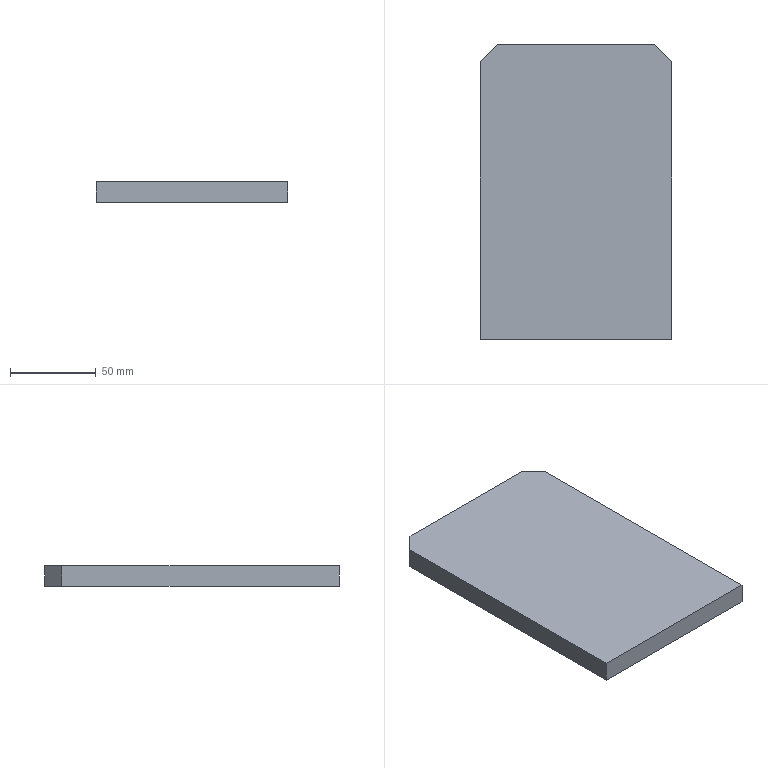Part | SolidWorks | features BaseBody 1 | 1 solid | 8 faces | box 112 x 172 x 12 mm | volume 229968 mm3 | plane 8
STEP:
#1=CARTESIAN_POINT('',(56.,-84.5,-6.));
#2=VERTEX_POINT('',#1);
#3=CARTESIAN_POINT('',(56.,-84.5,6.));
#4=VERTEX_POINT('',#3);
#5=CARTESIAN_POINT('',(56.,-84.5,6.));
#6=DIRECTION('',(0.,0.,1.));
#7=VECTOR('',#6,1000.);
#8=LINE('',#5,#7);
#9=EDGE_CURVE('',#2,#4,#8,.T.);
#10=ORIENTED_EDGE('',*,*,#9,.F.);
#11=CARTESIAN_POINT('',(56.,77.5,-6.));
#12=VERTEX_POINT('',#11);
#13=CARTESIAN_POINT('',(56.,77.5,-6.));
#14=DIRECTION('',(0.,1.,0.));
#15=VECTOR('',#14,1000.);
#16=LINE('',#13,#15);
#17=EDGE_CURVE('',#2,#12,#16,.T.);
#18=ORIENTED_EDGE('',*,*,#17,.T.);
#19=CARTESIAN_POINT('',(56.,77.5,6.));
#20=VERTEX_POINT('',#19);
#21=CARTESIAN_POINT('',(56.,77.5,6.));
#22=DIRECTION('',(0.,0.,-1.));
#23=VECTOR('',#22,1000.);
#24=LINE('',#21,#23);
#25=EDGE_CURVE('',#20,#12,#24,.T.);
#26=ORIENTED_EDGE('',*,*,#25,.F.);
#27=CARTESIAN_POINT('',(56.,77.5,6.));
#28=DIRECTION('',(0.,1.,0.));
#29=VECTOR('',#28,1000.);
#30=LINE('',#27,#29);
#31=EDGE_CURVE('',#4,#20,#30,.T.);
#32=ORIENTED_EDGE('',*,*,#31,.F.);
#33=EDGE_LOOP('',(#10,#18,#26,#32));
#34=FACE_OUTER_BOUND('',#33,.T.);
#35=CARTESIAN_POINT('',(56.,77.5,6.));
#36=DIRECTION('',(-1.,0.,0.));
#37=DIRECTION('',(0.,-1.,0.));
#38=AXIS2_PLACEMENT_3D('',#35,#36,#37);
#39=PLANE('',#38);
#40=ADVANCED_FACE('',(#34),#39,.F.);
#41=CARTESIAN_POINT('',(-56.,-84.5,6.));
#42=VERTEX_POINT('',#41);
#43=CARTESIAN_POINT('',(-56.,-84.5,-6.));
#44=VERTEX_POINT('',#43);
#45=CARTESIAN_POINT('',(-56.,-84.5,6.));
#46=DIRECTION('',(0.,0.,-1.));
#47=VECTOR('',#46,1000.);
#48=LINE('',#45,#47);
#49=EDGE_CURVE('',#42,#44,#48,.T.);
#50=ORIENTED_EDGE('',*,*,#49,.F.);
#51=CARTESIAN_POINT('',(-56.,77.5,6.));
#52=VERTEX_POINT('',#51);
#53=CARTESIAN_POINT('',(-56.,77.5,6.));
#54=DIRECTION('',(0.,-1.,0.));
#55=VECTOR('',#54,1000.);
#56=LINE('',#53,#55);
#57=EDGE_CURVE('',#52,#42,#56,.T.);
#58=ORIENTED_EDGE('',*,*,#57,.F.);
#59=CARTESIAN_POINT('',(-56.,77.5,-6.));
#60=VERTEX_POINT('',#59);
#61=CARTESIAN_POINT('',(-56.,77.5,6.));
#62=DIRECTION('',(0.,0.,-1.));
#63=VECTOR('',#62,1000.);
#64=LINE('',#61,#63);
#65=EDGE_CURVE('',#52,#60,#64,.T.);
#66=ORIENTED_EDGE('',*,*,#65,.T.);
#67=CARTESIAN_POINT('',(-56.,77.5,-6.));
#68=DIRECTION('',(0.,-1.,0.));
#69=VECTOR('',#68,1000.);
#70=LINE('',#67,#69);
#71=EDGE_CURVE('',#60,#44,#70,.T.);
#72=ORIENTED_EDGE('',*,*,#71,.T.);
#73=EDGE_LOOP('',(#50,#58,#66,#72));
#74=FACE_OUTER_BOUND('',#73,.T.);
#75=CARTESIAN_POINT('',(-56.,77.5,6.));
#76=DIRECTION('',(1.,0.,0.));
#77=DIRECTION('',(0.,1.,0.));
#78=AXIS2_PLACEMENT_3D('',#75,#76,#77);
#79=PLANE('',#78);
#80=ADVANCED_FACE('',(#74),#79,.F.);
#81=ORIENTED_EDGE('',*,*,#57,.T.);
#82=CARTESIAN_POINT('',(-70.,-84.5,6.));
#83=DIRECTION('',(-1.,0.,0.));
#84=VECTOR('',#83,1000.);
#85=LINE('',#82,#84);
#86=EDGE_CURVE('',#4,#42,#85,.T.);
#87=ORIENTED_EDGE('',*,*,#86,.F.);
#88=ORIENTED_EDGE('',*,*,#31,.T.);
#89=CARTESIAN_POINT('',(46.,87.5,6.));
#90=VERTEX_POINT('',#89);
#91=CARTESIAN_POINT('',(46.,87.5,6.));
#92=DIRECTION('',(-0.7071,0.7071,0.));
#93=VECTOR('',#92,1000.);
#94=LINE('',#91,#93);
#95=EDGE_CURVE('',#20,#90,#94,.T.);
#96=ORIENTED_EDGE('',*,*,#95,.T.);
#97=CARTESIAN_POINT('',(-46.,87.5,6.));
#98=VERTEX_POINT('',#97);
#99=CARTESIAN_POINT('',(-46.,87.5,6.));
#100=DIRECTION('',(-1.,0.,0.));
#101=VECTOR('',#100,1000.);
#102=LINE('',#99,#101);
#103=EDGE_CURVE('',#90,#98,#102,.T.);
#104=ORIENTED_EDGE('',*,*,#103,.T.);
#105=CARTESIAN_POINT('',(-56.,77.5,6.));
#106=DIRECTION('',(-0.7071,-0.7071,0.));
#107=VECTOR('',#106,1000.);
#108=LINE('',#105,#107);
#109=EDGE_CURVE('',#98,#52,#108,.T.);
#110=ORIENTED_EDGE('',*,*,#109,.T.);
#111=EDGE_LOOP('',(#81,#87,#88,#96,#104,#110));
#112=FACE_OUTER_BOUND('',#111,.T.);
#113=CARTESIAN_POINT('',(0.,0.,6.));
#114=DIRECTION('',(0.,0.,1.));
#115=DIRECTION('',(1.,0.,0.));
#116=AXIS2_PLACEMENT_3D('',#113,#114,#115);
#117=PLANE('',#116);
#118=ADVANCED_FACE('',(#112),#117,.T.);
#119=CARTESIAN_POINT('',(0.,-84.5,-6.));
#120=DIRECTION('',(1.,0.,0.));
#121=VECTOR('',#120,1000.);
#122=LINE('',#119,#121);
#123=EDGE_CURVE('',#44,#2,#122,.T.);
#124=ORIENTED_EDGE('',*,*,#123,.F.);
#125=ORIENTED_EDGE('',*,*,#71,.F.);
#126=CARTESIAN_POINT('',(-46.,87.5,-6.));
#127=VERTEX_POINT('',#126);
#128=CARTESIAN_POINT('',(-56.,77.5,-6.));
#129=DIRECTION('',(-0.7071,-0.7071,0.));
#130=VECTOR('',#129,1000.);
#131=LINE('',#128,#130);
#132=EDGE_CURVE('',#127,#60,#131,.T.);
#133=ORIENTED_EDGE('',*,*,#132,.F.);
#134=CARTESIAN_POINT('',(46.,87.5,-6.));
#135=VERTEX_POINT('',#134);
#136=CARTESIAN_POINT('',(-46.,87.5,-6.));
#137=DIRECTION('',(-1.,0.,0.));
#138=VECTOR('',#137,1000.);
#139=LINE('',#136,#138);
#140=EDGE_CURVE('',#135,#127,#139,.T.);
#141=ORIENTED_EDGE('',*,*,#140,.F.);
#142=CARTESIAN_POINT('',(46.,87.5,-6.));
#143=DIRECTION('',(-0.7071,0.7071,0.));
#144=VECTOR('',#143,1000.);
#145=LINE('',#142,#144);
#146=EDGE_CURVE('',#12,#135,#145,.T.);
#147=ORIENTED_EDGE('',*,*,#146,.F.);
#148=ORIENTED_EDGE('',*,*,#17,.F.);
#149=EDGE_LOOP('',(#124,#125,#133,#141,#147,#148));
#150=FACE_OUTER_BOUND('',#149,.T.);
#151=CARTESIAN_POINT('',(0.,0.,-6.));
#152=DIRECTION('',(0.,0.,1.));
#153=DIRECTION('',(1.,0.,0.));
#154=AXIS2_PLACEMENT_3D('',#151,#152,#153);
#155=PLANE('',#154);
#156=ADVANCED_FACE('',(#150),#155,.F.);
#157=ORIENTED_EDGE('',*,*,#146,.T.);
#158=CARTESIAN_POINT('',(46.,87.5,6.));
#159=DIRECTION('',(0.,0.,-1.));
#160=VECTOR('',#159,1000.);
#161=LINE('',#158,#160);
#162=EDGE_CURVE('',#90,#135,#161,.T.);
#163=ORIENTED_EDGE('',*,*,#162,.F.);
#164=ORIENTED_EDGE('',*,*,#95,.F.);
#165=ORIENTED_EDGE('',*,*,#25,.T.);
#166=EDGE_LOOP('',(#157,#163,#164,#165));
#167=FACE_OUTER_BOUND('',#166,.T.);
#168=CARTESIAN_POINT('',(46.,87.5,6.));
#169=DIRECTION('',(-0.7071,-0.7071,0.));
#170=DIRECTION('',(0.7071,-0.7071,0.));
#171=AXIS2_PLACEMENT_3D('',#168,#169,#170);
#172=PLANE('',#171);
#173=ADVANCED_FACE('',(#167),#172,.F.);
#174=ORIENTED_EDGE('',*,*,#140,.T.);
#175=CARTESIAN_POINT('',(-46.,87.5,6.));
#176=DIRECTION('',(0.,0.,-1.));
#177=VECTOR('',#176,1000.);
#178=LINE('',#175,#177);
#179=EDGE_CURVE('',#98,#127,#178,.T.);
#180=ORIENTED_EDGE('',*,*,#179,.F.);
#181=ORIENTED_EDGE('',*,*,#103,.F.);
#182=ORIENTED_EDGE('',*,*,#162,.T.);
#183=EDGE_LOOP('',(#174,#180,#181,#182));
#184=FACE_OUTER_BOUND('',#183,.T.);
#185=CARTESIAN_POINT('',(-46.,87.5,6.));
#186=DIRECTION('',(0.,-1.,0.));
#187=DIRECTION('',(0.,0.,-1.));
#188=AXIS2_PLACEMENT_3D('',#185,#186,#187);
#189=PLANE('',#188);
#190=ADVANCED_FACE('',(#184),#189,.F.);
#191=ORIENTED_EDGE('',*,*,#132,.T.);
#192=ORIENTED_EDGE('',*,*,#65,.F.);
#193=ORIENTED_EDGE('',*,*,#109,.F.);
#194=ORIENTED_EDGE('',*,*,#179,.T.);
#195=EDGE_LOOP('',(#191,#192,#193,#194));
#196=FACE_OUTER_BOUND('',#195,.T.);
#197=CARTESIAN_POINT('',(-56.,77.5,6.));
#198=DIRECTION('',(0.7071,-0.7071,0.));
#199=DIRECTION('',(0.7071,0.7071,0.));
#200=AXIS2_PLACEMENT_3D('',#197,#198,#199);
#201=PLANE('',#200);
#202=ADVANCED_FACE('',(#196),#201,.F.);
#203=ORIENTED_EDGE('',*,*,#9,.T.);
#204=ORIENTED_EDGE('',*,*,#86,.T.);
#205=ORIENTED_EDGE('',*,*,#49,.T.);
#206=ORIENTED_EDGE('',*,*,#123,.T.);
#207=EDGE_LOOP('',(#203,#204,#205,#206));
#208=FACE_OUTER_BOUND('',#207,.T.);
#209=CARTESIAN_POINT('',(0.,-84.5,-594.));
#210=DIRECTION('',(0.,-1.,0.));
#211=DIRECTION('',(1.,0.,0.));
#212=AXIS2_PLACEMENT_3D('',#209,#210,#211);
#213=PLANE('',#212);
#214=ADVANCED_FACE('',(#208),#213,.T.);
#215=CLOSED_SHELL('',(#40,#80,#118,#156,#173,#190,#202,#214));
#216=MANIFOLD_SOLID_BREP('',#215);
#217=CARTESIAN_POINT('',(0.,0.,0.));
#218=DIRECTION('',(0.,0.,1.));
#219=DIRECTION('',(1.,0.,0.));
#220=AXIS2_PLACEMENT_3D('',#217,#218,#219);
#221=(LENGTH_UNIT()NAMED_UNIT(*)SI_UNIT(.MILLI.,.METRE.));
#222=UNCERTAINTY_MEASURE_WITH_UNIT(LENGTH_MEASURE(0.00001),#221,'','');
#223=(NAMED_UNIT(*)PLANE_ANGLE_UNIT()SI_UNIT($,.RADIAN.));
#224=(NAMED_UNIT(*)SI_UNIT($,.STERADIAN.)SOLID_ANGLE_UNIT());
#225=(GEOMETRIC_REPRESENTATION_CONTEXT(3)GLOBAL_UNCERTAINTY_ASSIGNED_CONTEXT((#222))GLOBAL_UNIT_ASSIGNED_CONTEXT((#221,#223,#224))REPRESENTATION_CONTEXT('',''));
#226=ADVANCED_BREP_SHAPE_REPRESENTATION('',(#216,#220),#225);